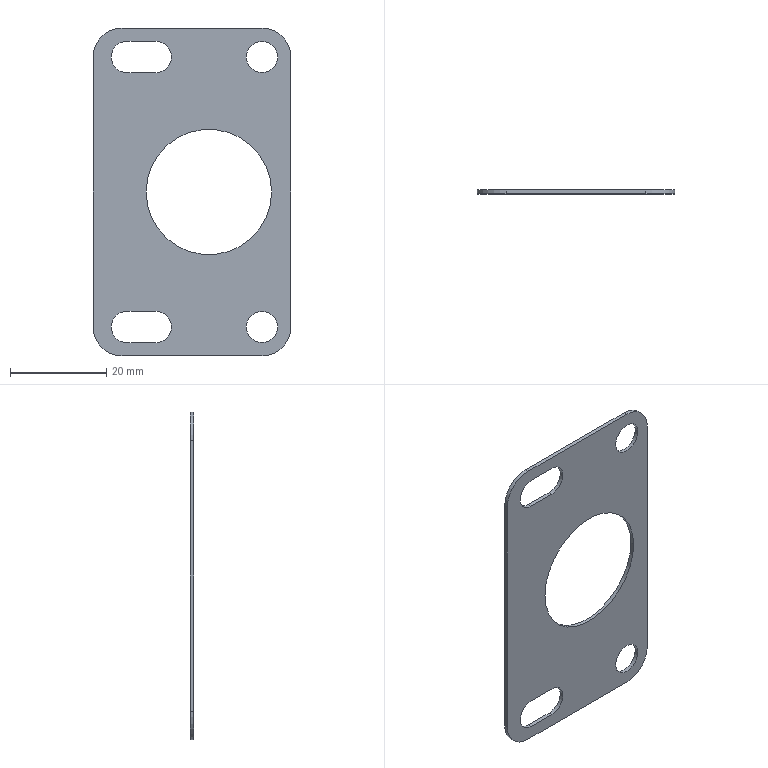Part | SolidWorks | features BaseBody 1 | 1 solid | 26 faces | box 41 x 0.8 x 68 mm | volume 1612 mm3 | cylinder 16 | plane 10 | commonest cylinder face diameters 6.5 x10 12 x4 26 x2
STEP:
#1=CARTESIAN_POINT('',(286.3,201.5,0.));
#2=VERTEX_POINT('',#1);
#3=CARTESIAN_POINT('',(312.3,201.5,0.));
#4=VERTEX_POINT('',#3);
#5=CARTESIAN_POINT('',(299.3,201.5,0.));
#6=DIRECTION('',(0.,-1.,0.));
#7=DIRECTION('',(1.,0.,0.));
#8=AXIS2_PLACEMENT_3D('',#5,#6,#7);
#9=CIRCLE('',#8,13.);
#10=EDGE_CURVE('',#2,#4,#9,.T.);
#11=ORIENTED_EDGE('',*,*,#10,.T.);
#12=CARTESIAN_POINT('',(312.3,202.3,0.));
#13=VERTEX_POINT('',#12);
#14=CARTESIAN_POINT('',(312.3,201.5,0.));
#15=DIRECTION('',(0.,1.,0.));
#16=VECTOR('',#15,1000.);
#17=LINE('',#14,#16);
#18=EDGE_CURVE('',#4,#13,#17,.T.);
#19=ORIENTED_EDGE('',*,*,#18,.T.);
#20=CARTESIAN_POINT('',(286.3,202.3,0.));
#21=VERTEX_POINT('',#20);
#22=CARTESIAN_POINT('',(299.3,202.3,0.));
#23=DIRECTION('',(0.,-1.,0.));
#24=DIRECTION('',(1.,0.,0.));
#25=AXIS2_PLACEMENT_3D('',#22,#23,#24);
#26=CIRCLE('',#25,13.);
#27=EDGE_CURVE('',#21,#13,#26,.T.);
#28=ORIENTED_EDGE('',*,*,#27,.F.);
#29=CARTESIAN_POINT('',(286.3,201.5,0.));
#30=DIRECTION('',(0.,1.,0.));
#31=VECTOR('',#30,1000.);
#32=LINE('',#29,#31);
#33=EDGE_CURVE('',#2,#21,#32,.T.);
#34=ORIENTED_EDGE('',*,*,#33,.F.);
#35=EDGE_LOOP('',(#11,#19,#28,#34));
#36=FACE_OUTER_BOUND('',#35,.T.);
#37=CARTESIAN_POINT('',(299.3,201.5,0.));
#38=DIRECTION('',(0.,1.,0.));
#39=DIRECTION('',(-1.,0.,0.));
#40=AXIS2_PLACEMENT_3D('',#37,#38,#39);
#41=CYLINDRICAL_SURFACE('',#40,13.);
#42=ADVANCED_FACE('',(#36),#41,.F.);
#43=CARTESIAN_POINT('',(282.3,201.5,31.25));
#44=VERTEX_POINT('',#43);
#45=CARTESIAN_POINT('',(279.05,201.5,28.));
#46=VERTEX_POINT('',#45);
#47=CARTESIAN_POINT('',(282.3,201.5,28.));
#48=DIRECTION('',(0.,-1.,0.));
#49=DIRECTION('',(-1.,0.,0.));
#50=AXIS2_PLACEMENT_3D('',#47,#48,#49);
#51=CIRCLE('',#50,3.25);
#52=EDGE_CURVE('',#44,#46,#51,.T.);
#53=ORIENTED_EDGE('',*,*,#52,.T.);
#54=CARTESIAN_POINT('',(279.05,202.3,28.));
#55=VERTEX_POINT('',#54);
#56=CARTESIAN_POINT('',(279.05,201.5,28.));
#57=DIRECTION('',(0.,1.,0.));
#58=VECTOR('',#57,1000.);
#59=LINE('',#56,#58);
#60=EDGE_CURVE('',#46,#55,#59,.T.);
#61=ORIENTED_EDGE('',*,*,#60,.T.);
#62=CARTESIAN_POINT('',(282.3,202.3,31.25));
#63=VERTEX_POINT('',#62);
#64=CARTESIAN_POINT('',(282.3,202.3,28.));
#65=DIRECTION('',(0.,-1.,0.));
#66=DIRECTION('',(-1.,0.,0.));
#67=AXIS2_PLACEMENT_3D('',#64,#65,#66);
#68=CIRCLE('',#67,3.25);
#69=EDGE_CURVE('',#63,#55,#68,.T.);
#70=ORIENTED_EDGE('',*,*,#69,.F.);
#71=CARTESIAN_POINT('',(282.3,201.5,31.25));
#72=DIRECTION('',(0.,1.,0.));
#73=VECTOR('',#72,1000.);
#74=LINE('',#71,#73);
#75=EDGE_CURVE('',#44,#63,#74,.T.);
#76=ORIENTED_EDGE('',*,*,#75,.F.);
#77=EDGE_LOOP('',(#53,#61,#70,#76));
#78=FACE_OUTER_BOUND('',#77,.T.);
#79=CARTESIAN_POINT('',(282.3,201.5,28.));
#80=DIRECTION('',(0.,1.,0.));
#81=DIRECTION('',(-1.,0.,0.));
#82=AXIS2_PLACEMENT_3D('',#79,#80,#81);
#83=CYLINDRICAL_SURFACE('',#82,3.25);
#84=ADVANCED_FACE('',(#78),#83,.F.);
#85=CARTESIAN_POINT('',(282.3,201.5,-24.75));
#86=VERTEX_POINT('',#85);
#87=CARTESIAN_POINT('',(279.05,201.5,-28.));
#88=VERTEX_POINT('',#87);
#89=CARTESIAN_POINT('',(282.3,201.5,-28.));
#90=DIRECTION('',(0.,-1.,0.));
#91=DIRECTION('',(1.,0.,0.));
#92=AXIS2_PLACEMENT_3D('',#89,#90,#91);
#93=CIRCLE('',#92,3.25);
#94=EDGE_CURVE('',#86,#88,#93,.T.);
#95=ORIENTED_EDGE('',*,*,#94,.T.);
#96=CARTESIAN_POINT('',(279.05,202.3,-28.));
#97=VERTEX_POINT('',#96);
#98=CARTESIAN_POINT('',(279.05,201.5,-28.));
#99=DIRECTION('',(0.,1.,0.));
#100=VECTOR('',#99,1000.);
#101=LINE('',#98,#100);
#102=EDGE_CURVE('',#88,#97,#101,.T.);
#103=ORIENTED_EDGE('',*,*,#102,.T.);
#104=CARTESIAN_POINT('',(282.3,202.3,-24.75));
#105=VERTEX_POINT('',#104);
#106=CARTESIAN_POINT('',(282.3,202.3,-28.));
#107=DIRECTION('',(0.,-1.,0.));
#108=DIRECTION('',(1.,0.,0.));
#109=AXIS2_PLACEMENT_3D('',#106,#107,#108);
#110=CIRCLE('',#109,3.25);
#111=EDGE_CURVE('',#105,#97,#110,.T.);
#112=ORIENTED_EDGE('',*,*,#111,.F.);
#113=CARTESIAN_POINT('',(282.3,201.5,-24.75));
#114=DIRECTION('',(0.,1.,0.));
#115=VECTOR('',#114,1000.);
#116=LINE('',#113,#115);
#117=EDGE_CURVE('',#86,#105,#116,.T.);
#118=ORIENTED_EDGE('',*,*,#117,.F.);
#119=EDGE_LOOP('',(#95,#103,#112,#118));
#120=FACE_OUTER_BOUND('',#119,.T.);
#121=CARTESIAN_POINT('',(282.3,201.5,-28.));
#122=DIRECTION('',(0.,1.,0.));
#123=DIRECTION('',(-1.,0.,0.));
#124=AXIS2_PLACEMENT_3D('',#121,#122,#123);
#125=CYLINDRICAL_SURFACE('',#124,3.25);
#126=ADVANCED_FACE('',(#120),#125,.F.);
#127=CARTESIAN_POINT('',(307.05,201.5,-28.));
#128=VERTEX_POINT('',#127);
#129=CARTESIAN_POINT('',(313.55,201.5,-28.));
#130=VERTEX_POINT('',#129);
#131=CARTESIAN_POINT('',(310.3,201.5,-28.));
#132=DIRECTION('',(0.,-1.,0.));
#133=DIRECTION('',(-1.,0.,0.));
#134=AXIS2_PLACEMENT_3D('',#131,#132,#133);
#135=CIRCLE('',#134,3.25);
#136=EDGE_CURVE('',#128,#130,#135,.T.);
#137=ORIENTED_EDGE('',*,*,#136,.T.);
#138=CARTESIAN_POINT('',(313.55,202.3,-28.));
#139=VERTEX_POINT('',#138);
#140=CARTESIAN_POINT('',(313.55,201.5,-28.));
#141=DIRECTION('',(0.,1.,0.));
#142=VECTOR('',#141,1000.);
#143=LINE('',#140,#142);
#144=EDGE_CURVE('',#130,#139,#143,.T.);
#145=ORIENTED_EDGE('',*,*,#144,.T.);
#146=CARTESIAN_POINT('',(307.05,202.3,-28.));
#147=VERTEX_POINT('',#146);
#148=CARTESIAN_POINT('',(310.3,202.3,-28.));
#149=DIRECTION('',(0.,-1.,0.));
#150=DIRECTION('',(-1.,0.,0.));
#151=AXIS2_PLACEMENT_3D('',#148,#149,#150);
#152=CIRCLE('',#151,3.25);
#153=EDGE_CURVE('',#147,#139,#152,.T.);
#154=ORIENTED_EDGE('',*,*,#153,.F.);
#155=CARTESIAN_POINT('',(307.05,201.5,-28.));
#156=DIRECTION('',(0.,1.,0.));
#157=VECTOR('',#156,1000.);
#158=LINE('',#155,#157);
#159=EDGE_CURVE('',#128,#147,#158,.T.);
#160=ORIENTED_EDGE('',*,*,#159,.F.);
#161=EDGE_LOOP('',(#137,#145,#154,#160));
#162=FACE_OUTER_BOUND('',#161,.T.);
#163=CARTESIAN_POINT('',(310.3,201.5,-28.));
#164=DIRECTION('',(0.,1.,0.));
#165=DIRECTION('',(-1.,0.,0.));
#166=AXIS2_PLACEMENT_3D('',#163,#164,#165);
#167=CYLINDRICAL_SURFACE('',#166,3.25);
#168=ADVANCED_FACE('',(#162),#167,.F.);
#169=CARTESIAN_POINT('',(307.05,201.5,28.));
#170=VERTEX_POINT('',#169);
#171=CARTESIAN_POINT('',(313.55,201.5,28.));
#172=VERTEX_POINT('',#171);
#173=CARTESIAN_POINT('',(310.3,201.5,28.));
#174=DIRECTION('',(0.,-1.,0.));
#175=DIRECTION('',(1.,0.,0.));
#176=AXIS2_PLACEMENT_3D('',#173,#174,#175);
#177=CIRCLE('',#176,3.25);
#178=EDGE_CURVE('',#170,#172,#177,.T.);
#179=ORIENTED_EDGE('',*,*,#178,.T.);
#180=CARTESIAN_POINT('',(313.55,202.3,28.));
#181=VERTEX_POINT('',#180);
#182=CARTESIAN_POINT('',(313.55,201.5,28.));
#183=DIRECTION('',(0.,1.,0.));
#184=VECTOR('',#183,1000.);
#185=LINE('',#182,#184);
#186=EDGE_CURVE('',#172,#181,#185,.T.);
#187=ORIENTED_EDGE('',*,*,#186,.T.);
#188=CARTESIAN_POINT('',(307.05,202.3,28.));
#189=VERTEX_POINT('',#188);
#190=CARTESIAN_POINT('',(310.3,202.3,28.));
#191=DIRECTION('',(0.,-1.,0.));
#192=DIRECTION('',(1.,0.,0.));
#193=AXIS2_PLACEMENT_3D('',#190,#191,#192);
#194=CIRCLE('',#193,3.25);
#195=EDGE_CURVE('',#189,#181,#194,.T.);
#196=ORIENTED_EDGE('',*,*,#195,.F.);
#197=CARTESIAN_POINT('',(307.05,201.5,28.));
#198=DIRECTION('',(0.,1.,0.));
#199=VECTOR('',#198,1000.);
#200=LINE('',#197,#199);
#201=EDGE_CURVE('',#170,#189,#200,.T.);
#202=ORIENTED_EDGE('',*,*,#201,.F.);
#203=EDGE_LOOP('',(#179,#187,#196,#202));
#204=FACE_OUTER_BOUND('',#203,.T.);
#205=CARTESIAN_POINT('',(310.3,201.5,28.));
#206=DIRECTION('',(0.,1.,0.));
#207=DIRECTION('',(-1.,0.,0.));
#208=AXIS2_PLACEMENT_3D('',#205,#206,#207);
#209=CYLINDRICAL_SURFACE('',#208,3.25);
#210=ADVANCED_FACE('',(#204),#209,.F.);
#211=CARTESIAN_POINT('',(288.3,201.5,31.25));
#212=VERTEX_POINT('',#211);
#213=CARTESIAN_POINT('',(282.3,201.5,31.25));
#214=DIRECTION('',(-1.,0.,0.));
#215=VECTOR('',#214,1000.);
#216=LINE('',#213,#215);
#217=EDGE_CURVE('',#212,#44,#216,.T.);
#218=ORIENTED_EDGE('',*,*,#217,.F.);
#219=CARTESIAN_POINT('',(288.3,201.5,24.75));
#220=VERTEX_POINT('',#219);
#221=CARTESIAN_POINT('',(288.3,201.5,28.));
#222=DIRECTION('',(0.,-1.,0.));
#223=DIRECTION('',(1.,0.,0.));
#224=AXIS2_PLACEMENT_3D('',#221,#222,#223);
#225=CIRCLE('',#224,3.25);
#226=EDGE_CURVE('',#220,#212,#225,.T.);
#227=ORIENTED_EDGE('',*,*,#226,.F.);
#228=CARTESIAN_POINT('',(282.3,201.5,24.75));
#229=VERTEX_POINT('',#228);
#230=CARTESIAN_POINT('',(282.3,201.5,24.75));
#231=DIRECTION('',(1.,0.,0.));
#232=VECTOR('',#231,1000.);
#233=LINE('',#230,#232);
#234=EDGE_CURVE('',#229,#220,#233,.T.);
#235=ORIENTED_EDGE('',*,*,#234,.F.);
#236=CARTESIAN_POINT('',(282.3,201.5,28.));
#237=DIRECTION('',(0.,-1.,0.));
#238=DIRECTION('',(-1.,0.,0.));
#239=AXIS2_PLACEMENT_3D('',#236,#237,#238);
#240=CIRCLE('',#239,3.25);
#241=EDGE_CURVE('',#46,#229,#240,.T.);
#242=ORIENTED_EDGE('',*,*,#241,.F.);
#243=ORIENTED_EDGE('',*,*,#52,.F.);
#244=EDGE_LOOP('',(#218,#227,#235,#242,#243));
#245=FACE_BOUND('',#244,.T.);
#246=ORIENTED_EDGE('',*,*,#136,.F.);
#247=CARTESIAN_POINT('',(310.3,201.5,-28.));
#248=DIRECTION('',(0.,-1.,0.));
#249=DIRECTION('',(-1.,0.,0.));
#250=AXIS2_PLACEMENT_3D('',#247,#248,#249);
#251=CIRCLE('',#250,3.25);
#252=EDGE_CURVE('',#130,#128,#251,.T.);
#253=ORIENTED_EDGE('',*,*,#252,.F.);
#254=EDGE_LOOP('',(#246,#253));
#255=FACE_BOUND('',#254,.T.);
#256=CARTESIAN_POINT('',(310.3,201.5,-34.));
#257=VERTEX_POINT('',#256);
#258=CARTESIAN_POINT('',(316.3,201.5,-28.));
#259=VERTEX_POINT('',#258);
#260=CARTESIAN_POINT('',(310.3,201.5,-28.));
#261=DIRECTION('',(0.,-1.,0.));
#262=DIRECTION('',(1.,0.,0.));
#263=AXIS2_PLACEMENT_3D('',#260,#261,#262);
#264=CIRCLE('',#263,6.);
#265=EDGE_CURVE('',#257,#259,#264,.T.);
#266=ORIENTED_EDGE('',*,*,#265,.T.);
#267=CARTESIAN_POINT('',(316.3,201.5,28.));
#268=VERTEX_POINT('',#267);
#269=CARTESIAN_POINT('',(316.3,201.5,28.));
#270=DIRECTION('',(0.,0.,1.));
#271=VECTOR('',#270,1000.);
#272=LINE('',#269,#271);
#273=EDGE_CURVE('',#259,#268,#272,.T.);
#274=ORIENTED_EDGE('',*,*,#273,.T.);
#275=CARTESIAN_POINT('',(310.3,201.5,34.));
#276=VERTEX_POINT('',#275);
#277=CARTESIAN_POINT('',(310.3,201.5,28.));
#278=DIRECTION('',(0.,-1.,0.));
#279=DIRECTION('',(-1.,0.,0.));
#280=AXIS2_PLACEMENT_3D('',#277,#278,#279);
#281=CIRCLE('',#280,6.);
#282=EDGE_CURVE('',#268,#276,#281,.T.);
#283=ORIENTED_EDGE('',*,*,#282,.T.);
#284=CARTESIAN_POINT('',(281.3,201.5,34.));
#285=VERTEX_POINT('',#284);
#286=CARTESIAN_POINT('',(281.3,201.5,34.));
#287=DIRECTION('',(-1.,0.,0.));
#288=VECTOR('',#287,1000.);
#289=LINE('',#286,#288);
#290=EDGE_CURVE('',#276,#285,#289,.T.);
#291=ORIENTED_EDGE('',*,*,#290,.T.);
#292=CARTESIAN_POINT('',(275.3,201.5,28.));
#293=VERTEX_POINT('',#292);
#294=CARTESIAN_POINT('',(281.3,201.5,28.));
#295=DIRECTION('',(0.,-1.,0.));
#296=DIRECTION('',(1.,0.,0.));
#297=AXIS2_PLACEMENT_3D('',#294,#295,#296);
#298=CIRCLE('',#297,6.);
#299=EDGE_CURVE('',#285,#293,#298,.T.);
#300=ORIENTED_EDGE('',*,*,#299,.T.);
#301=CARTESIAN_POINT('',(275.3,201.5,-28.));
#302=VERTEX_POINT('',#301);
#303=CARTESIAN_POINT('',(275.3,201.5,-28.));
#304=DIRECTION('',(0.,0.,-1.));
#305=VECTOR('',#304,1000.);
#306=LINE('',#303,#305);
#307=EDGE_CURVE('',#293,#302,#306,.T.);
#308=ORIENTED_EDGE('',*,*,#307,.T.);
#309=CARTESIAN_POINT('',(281.3,201.5,-34.));
#310=VERTEX_POINT('',#309);
#311=CARTESIAN_POINT('',(281.3,201.5,-28.));
#312=DIRECTION('',(0.,-1.,0.));
#313=DIRECTION('',(-1.,0.,0.));
#314=AXIS2_PLACEMENT_3D('',#311,#312,#313);
#315=CIRCLE('',#314,6.);
#316=EDGE_CURVE('',#302,#310,#315,.T.);
#317=ORIENTED_EDGE('',*,*,#316,.T.);
#318=CARTESIAN_POINT('',(310.3,201.5,-34.));
#319=DIRECTION('',(1.,0.,0.));
#320=VECTOR('',#319,1000.);
#321=LINE('',#318,#320);
#322=EDGE_CURVE('',#310,#257,#321,.T.);
#323=ORIENTED_EDGE('',*,*,#322,.T.);
#324=EDGE_LOOP('',(#266,#274,#283,#291,#300,#308,#317,#323));
#325=FACE_OUTER_BOUND('',#324,.T.);
#326=ORIENTED_EDGE('',*,*,#178,.F.);
#327=CARTESIAN_POINT('',(310.3,201.5,28.));
#328=DIRECTION('',(0.,-1.,0.));
#329=DIRECTION('',(1.,0.,0.));
#330=AXIS2_PLACEMENT_3D('',#327,#328,#329);
#331=CIRCLE('',#330,3.25);
#332=EDGE_CURVE('',#172,#170,#331,.T.);
#333=ORIENTED_EDGE('',*,*,#332,.F.);
#334=EDGE_LOOP('',(#326,#333));
#335=FACE_BOUND('',#334,.T.);
#336=CARTESIAN_POINT('',(288.3,201.5,-24.75));
#337=VERTEX_POINT('',#336);
#338=CARTESIAN_POINT('',(282.3,201.5,-24.75));
#339=DIRECTION('',(-1.,0.,0.));
#340=VECTOR('',#339,1000.);
#341=LINE('',#338,#340);
#342=EDGE_CURVE('',#337,#86,#341,.T.);
#343=ORIENTED_EDGE('',*,*,#342,.F.);
#344=CARTESIAN_POINT('',(288.3,201.5,-31.25));
#345=VERTEX_POINT('',#344);
#346=CARTESIAN_POINT('',(288.3,201.5,-28.));
#347=DIRECTION('',(0.,-1.,0.));
#348=DIRECTION('',(-1.,0.,0.));
#349=AXIS2_PLACEMENT_3D('',#346,#347,#348);
#350=CIRCLE('',#349,3.25);
#351=EDGE_CURVE('',#345,#337,#350,.T.);
#352=ORIENTED_EDGE('',*,*,#351,.F.);
#353=CARTESIAN_POINT('',(282.3,201.5,-31.25));
#354=VERTEX_POINT('',#353);
#355=CARTESIAN_POINT('',(282.3,201.5,-31.25));
#356=DIRECTION('',(1.,0.,0.));
#357=VECTOR('',#356,1000.);
#358=LINE('',#355,#357);
#359=EDGE_CURVE('',#354,#345,#358,.T.);
#360=ORIENTED_EDGE('',*,*,#359,.F.);
#361=CARTESIAN_POINT('',(282.3,201.5,-28.));
#362=DIRECTION('',(0.,-1.,0.));
#363=DIRECTION('',(1.,0.,0.));
#364=AXIS2_PLACEMENT_3D('',#361,#362,#363);
#365=CIRCLE('',#364,3.25);
#366=EDGE_CURVE('',#88,#354,#365,.T.);
#367=ORIENTED_EDGE('',*,*,#366,.F.);
#368=ORIENTED_EDGE('',*,*,#94,.F.);
#369=EDGE_LOOP('',(#343,#352,#360,#367,#368));
#370=FACE_BOUND('',#369,.T.);
#371=ORIENTED_EDGE('',*,*,#10,.F.);
#372=CARTESIAN_POINT('',(299.3,201.5,0.));
#373=DIRECTION('',(0.,-1.,0.));
#374=DIRECTION('',(1.,0.,0.));
#375=AXIS2_PLACEMENT_3D('',#372,#373,#374);
#376=CIRCLE('',#375,13.);
#377=EDGE_CURVE('',#4,#2,#376,.T.);
#378=ORIENTED_EDGE('',*,*,#377,.F.);
#379=EDGE_LOOP('',(#371,#378));
#380=FACE_BOUND('',#379,.T.);
#381=CARTESIAN_POINT('',(310.3,201.5,-28.));
#382=DIRECTION('',(0.,-1.,0.));
#383=DIRECTION('',(1.,0.,0.));
#384=AXIS2_PLACEMENT_3D('',#381,#382,#383);
#385=PLANE('',#384);
#386=ADVANCED_FACE('',(#245,#255,#325,#335,#370,#380),#385,.T.);
#387=CARTESIAN_POINT('',(288.3,202.3,24.75));
#388=VERTEX_POINT('',#387);
#389=CARTESIAN_POINT('',(288.3,202.3,31.25));
#390=VERTEX_POINT('',#389);
#391=CARTESIAN_POINT('',(288.3,202.3,28.));
#392=DIRECTION('',(0.,-1.,0.));
#393=DIRECTION('',(1.,0.,0.));
#394=AXIS2_PLACEMENT_3D('',#391,#392,#393);
#395=CIRCLE('',#394,3.25);
#396=EDGE_CURVE('',#388,#390,#395,.T.);
#397=ORIENTED_EDGE('',*,*,#396,.T.);
#398=CARTESIAN_POINT('',(282.3,202.3,31.25));
#399=DIRECTION('',(-1.,0.,0.));
#400=VECTOR('',#399,1000.);
#401=LINE('',#398,#400);
#402=EDGE_CURVE('',#390,#63,#401,.T.);
#403=ORIENTED_EDGE('',*,*,#402,.T.);
#404=ORIENTED_EDGE('',*,*,#69,.T.);
#405=CARTESIAN_POINT('',(282.3,202.3,24.75));
#406=VERTEX_POINT('',#405);
#407=CARTESIAN_POINT('',(282.3,202.3,28.));
#408=DIRECTION('',(0.,-1.,0.));
#409=DIRECTION('',(-1.,0.,0.));
#410=AXIS2_PLACEMENT_3D('',#407,#408,#409);
#411=CIRCLE('',#410,3.25);
#412=EDGE_CURVE('',#55,#406,#411,.T.);
#413=ORIENTED_EDGE('',*,*,#412,.T.);
#414=CARTESIAN_POINT('',(282.3,202.3,24.75));
#415=DIRECTION('',(1.,0.,0.));
#416=VECTOR('',#415,1000.);
#417=LINE('',#414,#416);
#418=EDGE_CURVE('',#406,#388,#417,.T.);
#419=ORIENTED_EDGE('',*,*,#418,.T.);
#420=EDGE_LOOP('',(#397,#403,#404,#413,#419));
#421=FACE_BOUND('',#420,.T.);
#422=ORIENTED_EDGE('',*,*,#153,.T.);
#423=CARTESIAN_POINT('',(310.3,202.3,-28.));
#424=DIRECTION('',(0.,-1.,0.));
#425=DIRECTION('',(-1.,0.,0.));
#426=AXIS2_PLACEMENT_3D('',#423,#424,#425);
#427=CIRCLE('',#426,3.25);
#428=EDGE_CURVE('',#139,#147,#427,.T.);
#429=ORIENTED_EDGE('',*,*,#428,.T.);
#430=EDGE_LOOP('',(#422,#429));
#431=FACE_BOUND('',#430,.T.);
#432=CARTESIAN_POINT('',(310.3,202.3,-34.));
#433=VERTEX_POINT('',#432);
#434=CARTESIAN_POINT('',(316.3,202.3,-28.));
#435=VERTEX_POINT('',#434);
#436=CARTESIAN_POINT('',(310.3,202.3,-28.));
#437=DIRECTION('',(0.,-1.,0.));
#438=DIRECTION('',(1.,0.,0.));
#439=AXIS2_PLACEMENT_3D('',#436,#437,#438);
#440=CIRCLE('',#439,6.);
#441=EDGE_CURVE('',#433,#435,#440,.T.);
#442=ORIENTED_EDGE('',*,*,#441,.F.);
#443=CARTESIAN_POINT('',(281.3,202.3,-34.));
#444=VERTEX_POINT('',#443);
#445=CARTESIAN_POINT('',(310.3,202.3,-34.));
#446=DIRECTION('',(1.,0.,0.));
#447=VECTOR('',#446,1000.);
#448=LINE('',#445,#447);
#449=EDGE_CURVE('',#444,#433,#448,.T.);
#450=ORIENTED_EDGE('',*,*,#449,.F.);
#451=CARTESIAN_POINT('',(275.3,202.3,-28.));
#452=VERTEX_POINT('',#451);
#453=CARTESIAN_POINT('',(281.3,202.3,-28.));
#454=DIRECTION('',(0.,-1.,0.));
#455=DIRECTION('',(-1.,0.,0.));
#456=AXIS2_PLACEMENT_3D('',#453,#454,#455);
#457=CIRCLE('',#456,6.);
#458=EDGE_CURVE('',#452,#444,#457,.T.);
#459=ORIENTED_EDGE('',*,*,#458,.F.);
#460=CARTESIAN_POINT('',(275.3,202.3,28.));
#461=VERTEX_POINT('',#460);
#462=CARTESIAN_POINT('',(275.3,202.3,-28.));
#463=DIRECTION('',(0.,0.,-1.));
#464=VECTOR('',#463,1000.);
#465=LINE('',#462,#464);
#466=EDGE_CURVE('',#461,#452,#465,.T.);
#467=ORIENTED_EDGE('',*,*,#466,.F.);
#468=CARTESIAN_POINT('',(281.3,202.3,34.));
#469=VERTEX_POINT('',#468);
#470=CARTESIAN_POINT('',(281.3,202.3,28.));
#471=DIRECTION('',(0.,-1.,0.));
#472=DIRECTION('',(1.,0.,0.));
#473=AXIS2_PLACEMENT_3D('',#470,#471,#472);
#474=CIRCLE('',#473,6.);
#475=EDGE_CURVE('',#469,#461,#474,.T.);
#476=ORIENTED_EDGE('',*,*,#475,.F.);
#477=CARTESIAN_POINT('',(310.3,202.3,34.));
#478=VERTEX_POINT('',#477);
#479=CARTESIAN_POINT('',(281.3,202.3,34.));
#480=DIRECTION('',(-1.,0.,0.));
#481=VECTOR('',#480,1000.);
#482=LINE('',#479,#481);
#483=EDGE_CURVE('',#478,#469,#482,.T.);
#484=ORIENTED_EDGE('',*,*,#483,.F.);
#485=CARTESIAN_POINT('',(316.3,202.3,28.));
#486=VERTEX_POINT('',#485);
#487=CARTESIAN_POINT('',(310.3,202.3,28.));
#488=DIRECTION('',(0.,-1.,0.));
#489=DIRECTION('',(-1.,0.,0.));
#490=AXIS2_PLACEMENT_3D('',#487,#488,#489);
#491=CIRCLE('',#490,6.);
#492=EDGE_CURVE('',#486,#478,#491,.T.);
#493=ORIENTED_EDGE('',*,*,#492,.F.);
#494=CARTESIAN_POINT('',(316.3,202.3,28.));
#495=DIRECTION('',(0.,0.,1.));
#496=VECTOR('',#495,1000.);
#497=LINE('',#494,#496);
#498=EDGE_CURVE('',#435,#486,#497,.T.);
#499=ORIENTED_EDGE('',*,*,#498,.F.);
#500=EDGE_LOOP('',(#442,#450,#459,#467,#476,#484,#493,#499));
#501=FACE_OUTER_BOUND('',#500,.T.);
#502=ORIENTED_EDGE('',*,*,#195,.T.);
#503=CARTESIAN_POINT('',(310.3,202.3,28.));
#504=DIRECTION('',(0.,-1.,0.));
#505=DIRECTION('',(1.,0.,0.));
#506=AXIS2_PLACEMENT_3D('',#503,#504,#505);
#507=CIRCLE('',#506,3.25);
#508=EDGE_CURVE('',#181,#189,#507,.T.);
#509=ORIENTED_EDGE('',*,*,#508,.T.);
#510=EDGE_LOOP('',(#502,#509));
#511=FACE_BOUND('',#510,.T.);
#512=CARTESIAN_POINT('',(288.3,202.3,-31.25));
#513=VERTEX_POINT('',#512);
#514=CARTESIAN_POINT('',(288.3,202.3,-24.75));
#515=VERTEX_POINT('',#514);
#516=CARTESIAN_POINT('',(288.3,202.3,-28.));
#517=DIRECTION('',(0.,-1.,0.));
#518=DIRECTION('',(-1.,0.,0.));
#519=AXIS2_PLACEMENT_3D('',#516,#517,#518);
#520=CIRCLE('',#519,3.25);
#521=EDGE_CURVE('',#513,#515,#520,.T.);
#522=ORIENTED_EDGE('',*,*,#521,.T.);
#523=CARTESIAN_POINT('',(282.3,202.3,-24.75));
#524=DIRECTION('',(-1.,0.,0.));
#525=VECTOR('',#524,1000.);
#526=LINE('',#523,#525);
#527=EDGE_CURVE('',#515,#105,#526,.T.);
#528=ORIENTED_EDGE('',*,*,#527,.T.);
#529=ORIENTED_EDGE('',*,*,#111,.T.);
#530=CARTESIAN_POINT('',(282.3,202.3,-31.25));
#531=VERTEX_POINT('',#530);
#532=CARTESIAN_POINT('',(282.3,202.3,-28.));
#533=DIRECTION('',(0.,-1.,0.));
#534=DIRECTION('',(1.,0.,0.));
#535=AXIS2_PLACEMENT_3D('',#532,#533,#534);
#536=CIRCLE('',#535,3.25);
#537=EDGE_CURVE('',#97,#531,#536,.T.);
#538=ORIENTED_EDGE('',*,*,#537,.T.);
#539=CARTESIAN_POINT('',(282.3,202.3,-31.25));
#540=DIRECTION('',(1.,0.,0.));
#541=VECTOR('',#540,1000.);
#542=LINE('',#539,#541);
#543=EDGE_CURVE('',#531,#513,#542,.T.);
#544=ORIENTED_EDGE('',*,*,#543,.T.);
#545=EDGE_LOOP('',(#522,#528,#529,#538,#544));
#546=FACE_BOUND('',#545,.T.);
#547=ORIENTED_EDGE('',*,*,#27,.T.);
#548=CARTESIAN_POINT('',(299.3,202.3,0.));
#549=DIRECTION('',(0.,-1.,0.));
#550=DIRECTION('',(1.,0.,0.));
#551=AXIS2_PLACEMENT_3D('',#548,#549,#550);
#552=CIRCLE('',#551,13.);
#553=EDGE_CURVE('',#13,#21,#552,.T.);
#554=ORIENTED_EDGE('',*,*,#553,.T.);
#555=EDGE_LOOP('',(#547,#554));
#556=FACE_BOUND('',#555,.T.);
#557=CARTESIAN_POINT('',(310.3,202.3,-28.));
#558=DIRECTION('',(0.,-1.,0.));
#559=DIRECTION('',(1.,0.,0.));
#560=AXIS2_PLACEMENT_3D('',#557,#558,#559);
#561=PLANE('',#560);
#562=ADVANCED_FACE('',(#421,#431,#501,#511,#546,#556),#561,.F.);
#563=ORIENTED_EDGE('',*,*,#441,.T.);
#564=CARTESIAN_POINT('',(316.3,201.5,-28.));
#565=DIRECTION('',(0.,1.,0.));
#566=VECTOR('',#565,1000.);
#567=LINE('',#564,#566);
#568=EDGE_CURVE('',#259,#435,#567,.T.);
#569=ORIENTED_EDGE('',*,*,#568,.F.);
#570=ORIENTED_EDGE('',*,*,#265,.F.);
#571=CARTESIAN_POINT('',(310.3,201.5,-34.));
#572=DIRECTION('',(0.,1.,0.));
#573=VECTOR('',#572,1000.);
#574=LINE('',#571,#573);
#575=EDGE_CURVE('',#257,#433,#574,.T.);
#576=ORIENTED_EDGE('',*,*,#575,.T.);
#577=EDGE_LOOP('',(#563,#569,#570,#576));
#578=FACE_OUTER_BOUND('',#577,.T.);
#579=CARTESIAN_POINT('',(310.3,201.5,-28.));
#580=DIRECTION('',(0.,1.,0.));
#581=DIRECTION('',(-1.,0.,0.));
#582=AXIS2_PLACEMENT_3D('',#579,#580,#581);
#583=CYLINDRICAL_SURFACE('',#582,6.);
#584=ADVANCED_FACE('',(#578),#583,.T.);
#585=ORIENTED_EDGE('',*,*,#498,.T.);
#586=CARTESIAN_POINT('',(316.3,201.5,28.));
#587=DIRECTION('',(0.,1.,0.));
#588=VECTOR('',#587,1000.);
#589=LINE('',#586,#588);
#590=EDGE_CURVE('',#268,#486,#589,.T.);
#591=ORIENTED_EDGE('',*,*,#590,.F.);
#592=ORIENTED_EDGE('',*,*,#273,.F.);
#593=ORIENTED_EDGE('',*,*,#568,.T.);
#594=EDGE_LOOP('',(#585,#591,#592,#593));
#595=FACE_OUTER_BOUND('',#594,.T.);
#596=CARTESIAN_POINT('',(316.3,201.5,28.));
#597=DIRECTION('',(-1.,0.,0.));
#598=DIRECTION('',(0.,-1.,0.));
#599=AXIS2_PLACEMENT_3D('',#596,#597,#598);
#600=PLANE('',#599);
#601=ADVANCED_FACE('',(#595),#600,.F.);
#602=ORIENTED_EDGE('',*,*,#492,.T.);
#603=CARTESIAN_POINT('',(310.3,201.5,34.));
#604=DIRECTION('',(0.,1.,0.));
#605=VECTOR('',#604,1000.);
#606=LINE('',#603,#605);
#607=EDGE_CURVE('',#276,#478,#606,.T.);
#608=ORIENTED_EDGE('',*,*,#607,.F.);
#609=ORIENTED_EDGE('',*,*,#282,.F.);
#610=ORIENTED_EDGE('',*,*,#590,.T.);
#611=EDGE_LOOP('',(#602,#608,#609,#610));
#612=FACE_OUTER_BOUND('',#611,.T.);
#613=CARTESIAN_POINT('',(310.3,201.5,28.));
#614=DIRECTION('',(0.,1.,0.));
#615=DIRECTION('',(-1.,0.,0.));
#616=AXIS2_PLACEMENT_3D('',#613,#614,#615);
#617=CYLINDRICAL_SURFACE('',#616,6.);
#618=ADVANCED_FACE('',(#612),#617,.T.);
#619=ORIENTED_EDGE('',*,*,#483,.T.);
#620=CARTESIAN_POINT('',(281.3,201.5,34.));
#621=DIRECTION('',(0.,1.,0.));
#622=VECTOR('',#621,1000.);
#623=LINE('',#620,#622);
#624=EDGE_CURVE('',#285,#469,#623,.T.);
#625=ORIENTED_EDGE('',*,*,#624,.F.);
#626=ORIENTED_EDGE('',*,*,#290,.F.);
#627=ORIENTED_EDGE('',*,*,#607,.T.);
#628=EDGE_LOOP('',(#619,#625,#626,#627));
#629=FACE_OUTER_BOUND('',#628,.T.);
#630=CARTESIAN_POINT('',(281.3,201.5,34.));
#631=DIRECTION('',(0.,0.,-1.));
#632=DIRECTION('',(1.,0.,0.));
#633=AXIS2_PLACEMENT_3D('',#630,#631,#632);
#634=PLANE('',#633);
#635=ADVANCED_FACE('',(#629),#634,.F.);
#636=ORIENTED_EDGE('',*,*,#475,.T.);
#637=CARTESIAN_POINT('',(275.3,201.5,28.));
#638=DIRECTION('',(0.,1.,0.));
#639=VECTOR('',#638,1000.);
#640=LINE('',#637,#639);
#641=EDGE_CURVE('',#293,#461,#640,.T.);
#642=ORIENTED_EDGE('',*,*,#641,.F.);
#643=ORIENTED_EDGE('',*,*,#299,.F.);
#644=ORIENTED_EDGE('',*,*,#624,.T.);
#645=EDGE_LOOP('',(#636,#642,#643,#644));
#646=FACE_OUTER_BOUND('',#645,.T.);
#647=CARTESIAN_POINT('',(281.3,201.5,28.));
#648=DIRECTION('',(0.,1.,0.));
#649=DIRECTION('',(-1.,0.,0.));
#650=AXIS2_PLACEMENT_3D('',#647,#648,#649);
#651=CYLINDRICAL_SURFACE('',#650,6.);
#652=ADVANCED_FACE('',(#646),#651,.T.);
#653=ORIENTED_EDGE('',*,*,#466,.T.);
#654=CARTESIAN_POINT('',(275.3,201.5,-28.));
#655=DIRECTION('',(0.,1.,0.));
#656=VECTOR('',#655,1000.);
#657=LINE('',#654,#656);
#658=EDGE_CURVE('',#302,#452,#657,.T.);
#659=ORIENTED_EDGE('',*,*,#658,.F.);
#660=ORIENTED_EDGE('',*,*,#307,.F.);
#661=ORIENTED_EDGE('',*,*,#641,.T.);
#662=EDGE_LOOP('',(#653,#659,#660,#661));
#663=FACE_OUTER_BOUND('',#662,.T.);
#664=CARTESIAN_POINT('',(275.3,201.5,-28.));
#665=DIRECTION('',(1.,0.,0.));
#666=DIRECTION('',(0.,1.,0.));
#667=AXIS2_PLACEMENT_3D('',#664,#665,#666);
#668=PLANE('',#667);
#669=ADVANCED_FACE('',(#663),#668,.F.);
#670=ORIENTED_EDGE('',*,*,#458,.T.);
#671=CARTESIAN_POINT('',(281.3,201.5,-34.));
#672=DIRECTION('',(0.,1.,0.));
#673=VECTOR('',#672,1000.);
#674=LINE('',#671,#673);
#675=EDGE_CURVE('',#310,#444,#674,.T.);
#676=ORIENTED_EDGE('',*,*,#675,.F.);
#677=ORIENTED_EDGE('',*,*,#316,.F.);
#678=ORIENTED_EDGE('',*,*,#658,.T.);
#679=EDGE_LOOP('',(#670,#676,#677,#678));
#680=FACE_OUTER_BOUND('',#679,.T.);
#681=CARTESIAN_POINT('',(281.3,201.5,-28.));
#682=DIRECTION('',(0.,1.,0.));
#683=DIRECTION('',(-1.,0.,0.));
#684=AXIS2_PLACEMENT_3D('',#681,#682,#683);
#685=CYLINDRICAL_SURFACE('',#684,6.);
#686=ADVANCED_FACE('',(#680),#685,.T.);
#687=ORIENTED_EDGE('',*,*,#449,.T.);
#688=ORIENTED_EDGE('',*,*,#575,.F.);
#689=ORIENTED_EDGE('',*,*,#322,.F.);
#690=ORIENTED_EDGE('',*,*,#675,.T.);
#691=EDGE_LOOP('',(#687,#688,#689,#690));
#692=FACE_OUTER_BOUND('',#691,.T.);
#693=CARTESIAN_POINT('',(310.3,201.5,-34.));
#694=DIRECTION('',(0.,0.,1.));
#695=DIRECTION('',(-1.,0.,0.));
#696=AXIS2_PLACEMENT_3D('',#693,#694,#695);
#697=PLANE('',#696);
#698=ADVANCED_FACE('',(#692),#697,.F.);
#699=ORIENTED_EDGE('',*,*,#186,.F.);
#700=ORIENTED_EDGE('',*,*,#332,.T.);
#701=ORIENTED_EDGE('',*,*,#201,.T.);
#702=ORIENTED_EDGE('',*,*,#508,.F.);
#703=EDGE_LOOP('',(#699,#700,#701,#702));
#704=FACE_OUTER_BOUND('',#703,.T.);
#705=CARTESIAN_POINT('',(310.3,201.5,28.));
#706=DIRECTION('',(0.,1.,0.));
#707=DIRECTION('',(-1.,0.,0.));
#708=AXIS2_PLACEMENT_3D('',#705,#706,#707);
#709=CYLINDRICAL_SURFACE('',#708,3.25);
#710=ADVANCED_FACE('',(#704),#709,.F.);
#711=ORIENTED_EDGE('',*,*,#144,.F.);
#712=ORIENTED_EDGE('',*,*,#252,.T.);
#713=ORIENTED_EDGE('',*,*,#159,.T.);
#714=ORIENTED_EDGE('',*,*,#428,.F.);
#715=EDGE_LOOP('',(#711,#712,#713,#714));
#716=FACE_OUTER_BOUND('',#715,.T.);
#717=CARTESIAN_POINT('',(310.3,201.5,-28.));
#718=DIRECTION('',(0.,1.,0.));
#719=DIRECTION('',(-1.,0.,0.));
#720=AXIS2_PLACEMENT_3D('',#717,#718,#719);
#721=CYLINDRICAL_SURFACE('',#720,3.25);
#722=ADVANCED_FACE('',(#716),#721,.F.);
#723=ORIENTED_EDGE('',*,*,#521,.F.);
#724=CARTESIAN_POINT('',(288.3,201.5,-31.25));
#725=DIRECTION('',(0.,1.,0.));
#726=VECTOR('',#725,1000.);
#727=LINE('',#724,#726);
#728=EDGE_CURVE('',#345,#513,#727,.T.);
#729=ORIENTED_EDGE('',*,*,#728,.F.);
#730=ORIENTED_EDGE('',*,*,#351,.T.);
#731=CARTESIAN_POINT('',(288.3,201.5,-24.75));
#732=DIRECTION('',(0.,1.,0.));
#733=VECTOR('',#732,1000.);
#734=LINE('',#731,#733);
#735=EDGE_CURVE('',#337,#515,#734,.T.);
#736=ORIENTED_EDGE('',*,*,#735,.T.);
#737=EDGE_LOOP('',(#723,#729,#730,#736));
#738=FACE_OUTER_BOUND('',#737,.T.);
#739=CARTESIAN_POINT('',(288.3,201.5,-28.));
#740=DIRECTION('',(0.,1.,0.));
#741=DIRECTION('',(-1.,0.,0.));
#742=AXIS2_PLACEMENT_3D('',#739,#740,#741);
#743=CYLINDRICAL_SURFACE('',#742,3.25);
#744=ADVANCED_FACE('',(#738),#743,.F.);
#745=ORIENTED_EDGE('',*,*,#527,.F.);
#746=ORIENTED_EDGE('',*,*,#735,.F.);
#747=ORIENTED_EDGE('',*,*,#342,.T.);
#748=ORIENTED_EDGE('',*,*,#117,.T.);
#749=EDGE_LOOP('',(#745,#746,#747,#748));
#750=FACE_OUTER_BOUND('',#749,.T.);
#751=CARTESIAN_POINT('',(282.3,201.5,-24.75));
#752=DIRECTION('',(0.,0.,-1.));
#753=DIRECTION('',(0.,1.,0.));
#754=AXIS2_PLACEMENT_3D('',#751,#752,#753);
#755=PLANE('',#754);
#756=ADVANCED_FACE('',(#750),#755,.T.);
#757=ORIENTED_EDGE('',*,*,#102,.F.);
#758=ORIENTED_EDGE('',*,*,#366,.T.);
#759=CARTESIAN_POINT('',(282.3,201.5,-31.25));
#760=DIRECTION('',(0.,1.,0.));
#761=VECTOR('',#760,1000.);
#762=LINE('',#759,#761);
#763=EDGE_CURVE('',#354,#531,#762,.T.);
#764=ORIENTED_EDGE('',*,*,#763,.T.);
#765=ORIENTED_EDGE('',*,*,#537,.F.);
#766=EDGE_LOOP('',(#757,#758,#764,#765));
#767=FACE_OUTER_BOUND('',#766,.T.);
#768=CARTESIAN_POINT('',(282.3,201.5,-28.));
#769=DIRECTION('',(0.,1.,0.));
#770=DIRECTION('',(-1.,0.,0.));
#771=AXIS2_PLACEMENT_3D('',#768,#769,#770);
#772=CYLINDRICAL_SURFACE('',#771,3.25);
#773=ADVANCED_FACE('',(#767),#772,.F.);
#774=ORIENTED_EDGE('',*,*,#543,.F.);
#775=ORIENTED_EDGE('',*,*,#763,.F.);
#776=ORIENTED_EDGE('',*,*,#359,.T.);
#777=ORIENTED_EDGE('',*,*,#728,.T.);
#778=EDGE_LOOP('',(#774,#775,#776,#777));
#779=FACE_OUTER_BOUND('',#778,.T.);
#780=CARTESIAN_POINT('',(282.3,201.5,-31.25));
#781=DIRECTION('',(0.,0.,1.));
#782=DIRECTION('',(0.,-1.,0.));
#783=AXIS2_PLACEMENT_3D('',#780,#781,#782);
#784=PLANE('',#783);
#785=ADVANCED_FACE('',(#779),#784,.T.);
#786=ORIENTED_EDGE('',*,*,#396,.F.);
#787=CARTESIAN_POINT('',(288.3,201.5,24.75));
#788=DIRECTION('',(0.,1.,0.));
#789=VECTOR('',#788,1000.);
#790=LINE('',#787,#789);
#791=EDGE_CURVE('',#220,#388,#790,.T.);
#792=ORIENTED_EDGE('',*,*,#791,.F.);
#793=ORIENTED_EDGE('',*,*,#226,.T.);
#794=CARTESIAN_POINT('',(288.3,201.5,31.25));
#795=DIRECTION('',(0.,1.,0.));
#796=VECTOR('',#795,1000.);
#797=LINE('',#794,#796);
#798=EDGE_CURVE('',#212,#390,#797,.T.);
#799=ORIENTED_EDGE('',*,*,#798,.T.);
#800=EDGE_LOOP('',(#786,#792,#793,#799));
#801=FACE_OUTER_BOUND('',#800,.T.);
#802=CARTESIAN_POINT('',(288.3,201.5,28.));
#803=DIRECTION('',(0.,1.,0.));
#804=DIRECTION('',(-1.,0.,0.));
#805=AXIS2_PLACEMENT_3D('',#802,#803,#804);
#806=CYLINDRICAL_SURFACE('',#805,3.25);
#807=ADVANCED_FACE('',(#801),#806,.F.);
#808=ORIENTED_EDGE('',*,*,#402,.F.);
#809=ORIENTED_EDGE('',*,*,#798,.F.);
#810=ORIENTED_EDGE('',*,*,#217,.T.);
#811=ORIENTED_EDGE('',*,*,#75,.T.);
#812=EDGE_LOOP('',(#808,#809,#810,#811));
#813=FACE_OUTER_BOUND('',#812,.T.);
#814=CARTESIAN_POINT('',(282.3,201.5,31.25));
#815=DIRECTION('',(0.,0.,-1.));
#816=DIRECTION('',(0.,1.,0.));
#817=AXIS2_PLACEMENT_3D('',#814,#815,#816);
#818=PLANE('',#817);
#819=ADVANCED_FACE('',(#813),#818,.T.);
#820=ORIENTED_EDGE('',*,*,#60,.F.);
#821=ORIENTED_EDGE('',*,*,#241,.T.);
#822=CARTESIAN_POINT('',(282.3,201.5,24.75));
#823=DIRECTION('',(0.,1.,0.));
#824=VECTOR('',#823,1000.);
#825=LINE('',#822,#824);
#826=EDGE_CURVE('',#229,#406,#825,.T.);
#827=ORIENTED_EDGE('',*,*,#826,.T.);
#828=ORIENTED_EDGE('',*,*,#412,.F.);
#829=EDGE_LOOP('',(#820,#821,#827,#828));
#830=FACE_OUTER_BOUND('',#829,.T.);
#831=CARTESIAN_POINT('',(282.3,201.5,28.));
#832=DIRECTION('',(0.,1.,0.));
#833=DIRECTION('',(-1.,0.,0.));
#834=AXIS2_PLACEMENT_3D('',#831,#832,#833);
#835=CYLINDRICAL_SURFACE('',#834,3.25);
#836=ADVANCED_FACE('',(#830),#835,.F.);
#837=ORIENTED_EDGE('',*,*,#418,.F.);
#838=ORIENTED_EDGE('',*,*,#826,.F.);
#839=ORIENTED_EDGE('',*,*,#234,.T.);
#840=ORIENTED_EDGE('',*,*,#791,.T.);
#841=EDGE_LOOP('',(#837,#838,#839,#840));
#842=FACE_OUTER_BOUND('',#841,.T.);
#843=CARTESIAN_POINT('',(282.3,201.5,24.75));
#844=DIRECTION('',(0.,0.,1.));
#845=DIRECTION('',(0.,-1.,0.));
#846=AXIS2_PLACEMENT_3D('',#843,#844,#845);
#847=PLANE('',#846);
#848=ADVANCED_FACE('',(#842),#847,.T.);
#849=ORIENTED_EDGE('',*,*,#18,.F.);
#850=ORIENTED_EDGE('',*,*,#377,.T.);
#851=ORIENTED_EDGE('',*,*,#33,.T.);
#852=ORIENTED_EDGE('',*,*,#553,.F.);
#853=EDGE_LOOP('',(#849,#850,#851,#852));
#854=FACE_OUTER_BOUND('',#853,.T.);
#855=CARTESIAN_POINT('',(299.3,201.5,0.));
#856=DIRECTION('',(0.,1.,0.));
#857=DIRECTION('',(-1.,0.,0.));
#858=AXIS2_PLACEMENT_3D('',#855,#856,#857);
#859=CYLINDRICAL_SURFACE('',#858,13.);
#860=ADVANCED_FACE('',(#854),#859,.F.);
#861=CLOSED_SHELL('',(#42,#84,#126,#168,#210,#386,#562,#584,#601,#618,#635,#652,#669,#686,#698,#710,#722,#744,#756,#773,#785,#807,#819,#836,#848,#860));
#862=MANIFOLD_SOLID_BREP('',#861);
#863=CARTESIAN_POINT('',(0.,0.,0.));
#864=DIRECTION('',(0.,0.,1.));
#865=DIRECTION('',(1.,0.,0.));
#866=AXIS2_PLACEMENT_3D('',#863,#864,#865);
#867=(LENGTH_UNIT()NAMED_UNIT(*)SI_UNIT(.MILLI.,.METRE.));
#868=UNCERTAINTY_MEASURE_WITH_UNIT(LENGTH_MEASURE(0.00001),#867,'','');
#869=(NAMED_UNIT(*)PLANE_ANGLE_UNIT()SI_UNIT($,.RADIAN.));
#870=(NAMED_UNIT(*)SI_UNIT($,.STERADIAN.)SOLID_ANGLE_UNIT());
#871=(GEOMETRIC_REPRESENTATION_CONTEXT(3)GLOBAL_UNCERTAINTY_ASSIGNED_CONTEXT((#868))GLOBAL_UNIT_ASSIGNED_CONTEXT((#867,#869,#870))REPRESENTATION_CONTEXT('',''));
#872=ADVANCED_BREP_SHAPE_REPRESENTATION('',(#862,#866),#871);